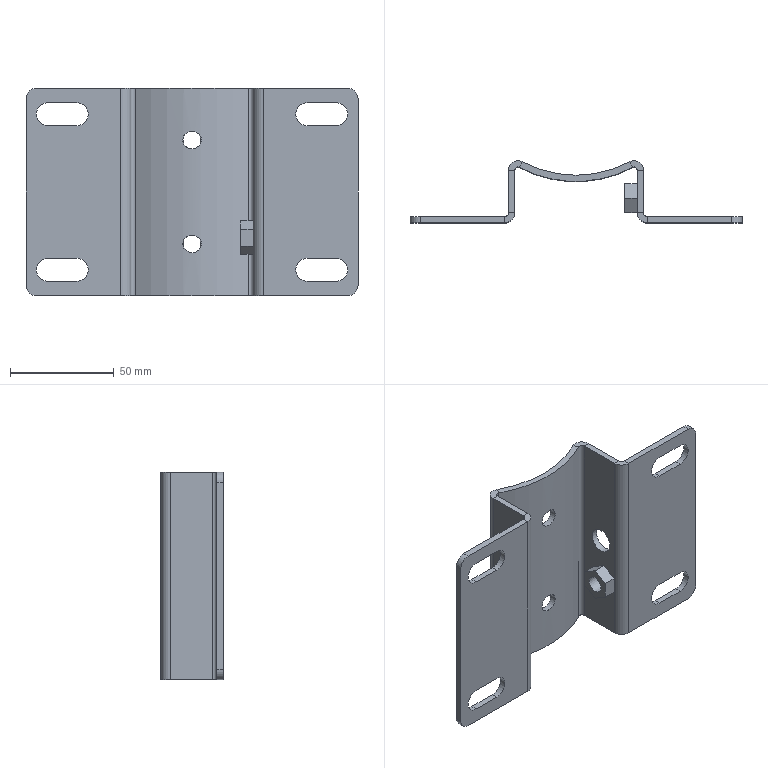Part | STEP file | 6100601 | 1 solid | 71 faces | box 160 x 30 x 100 mm | volume 59957 mm3 | plane 44 | cylinder 25 | spline 2 | commonest cylinder face diameters 11 x8 10 x7 3 x2 4 x2 9 x2 8 x1